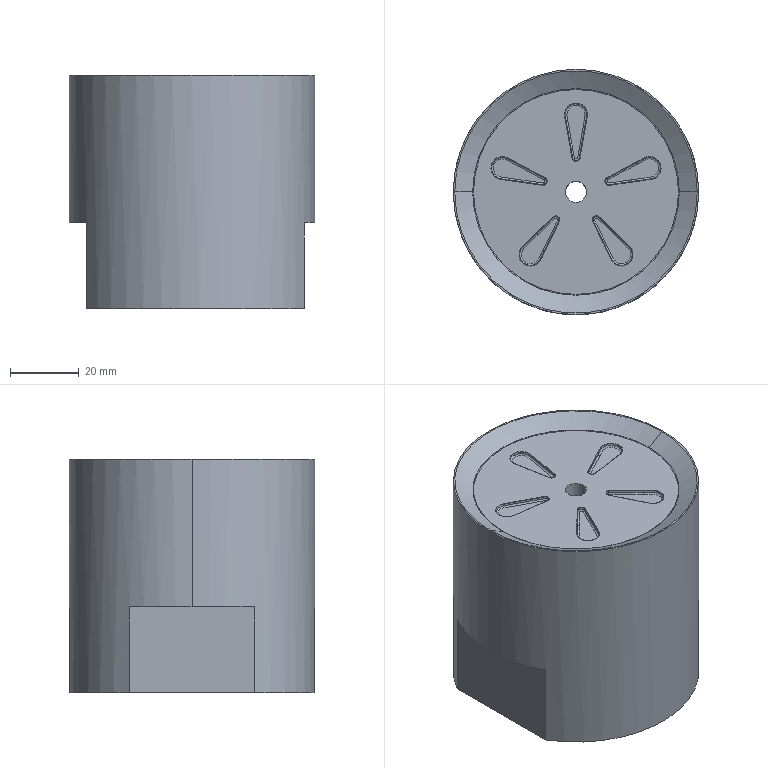Part | SolidWorks | features BaseBody 1 | 1 solid | 65 faces | box 71.5 x 71.5 x 68 mm | volume 251078 mm3 | spline 30 | plane 13 | cone 10 | cylinder 10 | torus 2 | commonest cylinder face diameters 6.806 x4 6.201 x2 10.505 x2 71.5 x2